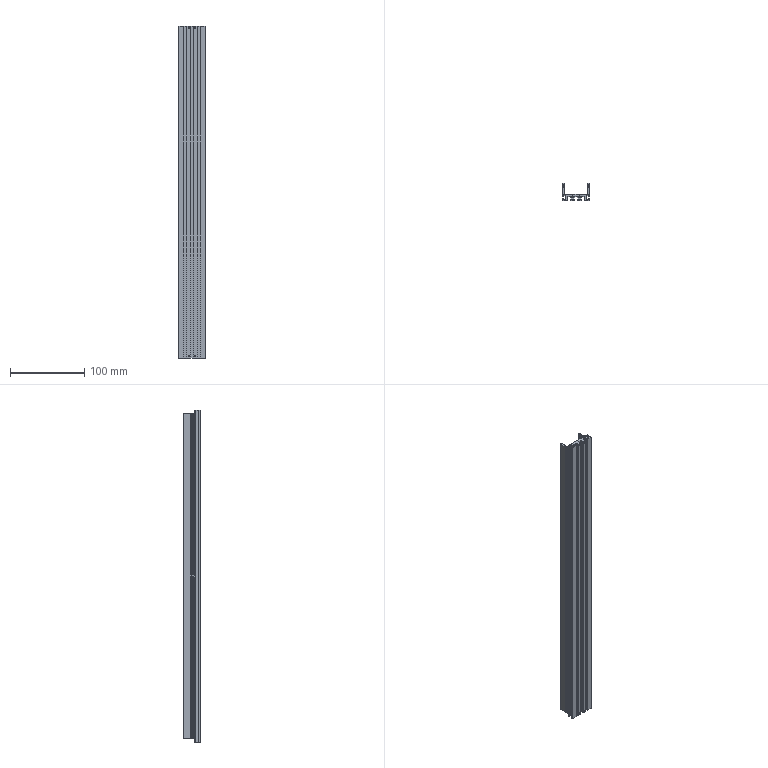Part | SolidWorks | features BaseBody 1 | 1 solid | 178 faces | box 36 x 22.6 x 446 mm | volume 102225 mm3 | plane 136 | cylinder 34 | cone 8 | commonest cylinder face diameters 0.6 x24 1.6 x8 2 x2